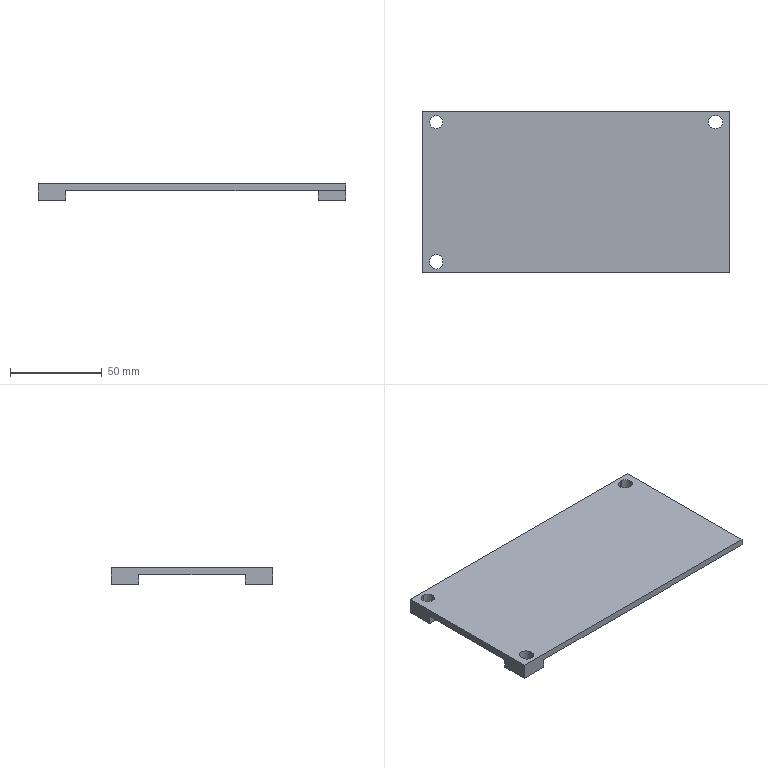Part | NX | 1 solid | 29 faces | box 168 x 88.2 x 8.8 mm | volume 57917 mm3 | plane 22 | cylinder 7 | commonest cylinder face diameters 7.17 x7
STEP:
#1=CARTESIAN_POINT('',(76.615,34.515,-8.8));
#2=VERTEX_POINT('',#1);
#3=CARTESIAN_POINT('',(76.615,34.515,0.));
#4=VERTEX_POINT('',#3);
#5=CARTESIAN_POINT('',(76.615,34.515,-8.8));
#6=DIRECTION('',(0.,0.,1.));
#7=VECTOR('',#6,1000.);
#8=LINE('',#5,#7);
#9=EDGE_CURVE('',#2,#4,#8,.T.);
#10=ORIENTED_EDGE('',*,*,#9,.T.);
#11=CARTESIAN_POINT('',(76.615,41.685,0.));
#12=VERTEX_POINT('',#11);
#13=CARTESIAN_POINT('',(76.615,38.1,0.));
#14=DIRECTION('',(0.,0.,-1.));
#15=DIRECTION('',(0.,1.,0.));
#16=AXIS2_PLACEMENT_3D('',#13,#14,#15);
#17=CIRCLE('',#16,3.585);
#18=EDGE_CURVE('',#12,#4,#17,.T.);
#19=ORIENTED_EDGE('',*,*,#18,.F.);
#20=CARTESIAN_POINT('',(76.615,41.685,-8.8));
#21=VERTEX_POINT('',#20);
#22=CARTESIAN_POINT('',(76.615,41.685,0.));
#23=DIRECTION('',(0.,0.,-1.));
#24=VECTOR('',#23,1000.);
#25=LINE('',#22,#24);
#26=EDGE_CURVE('',#12,#21,#25,.T.);
#27=ORIENTED_EDGE('',*,*,#26,.T.);
#28=CARTESIAN_POINT('',(76.615,38.1,-8.8));
#29=DIRECTION('',(0.,0.,1.));
#30=DIRECTION('',(0.,-1.,0.));
#31=AXIS2_PLACEMENT_3D('',#28,#29,#30);
#32=CIRCLE('',#31,3.585);
#33=EDGE_CURVE('',#2,#21,#32,.T.);
#34=ORIENTED_EDGE('',*,*,#33,.F.);
#35=EDGE_LOOP('',(#10,#19,#27,#34));
#36=FACE_BOUND('',#35,.T.);
#37=CARTESIAN_POINT('',(76.615,38.1,0.));
#38=DIRECTION('',(0.,0.,-1.));
#39=DIRECTION('',(0.,1.,0.));
#40=AXIS2_PLACEMENT_3D('',#37,#38,#39);
#41=CYLINDRICAL_SURFACE('',#40,3.585);
#42=ADVANCED_FACE('',(#36),#41,.F.);
#43=CARTESIAN_POINT('',(69.,29.1,-8.8));
#44=VERTEX_POINT('',#43);
#45=CARTESIAN_POINT('',(69.,44.1,-8.8));
#46=VERTEX_POINT('',#45);
#47=CARTESIAN_POINT('',(69.,29.1,-8.8));
#48=DIRECTION('',(0.,1.,0.));
#49=VECTOR('',#48,1000.);
#50=LINE('',#47,#49);
#51=EDGE_CURVE('',#44,#46,#50,.T.);
#52=ORIENTED_EDGE('',*,*,#51,.T.);
#53=CARTESIAN_POINT('',(84.,44.1,-8.8));
#54=VERTEX_POINT('',#53);
#55=CARTESIAN_POINT('',(84.,44.1,-8.8));
#56=DIRECTION('',(-1.,0.,0.));
#57=VECTOR('',#56,1000.);
#58=LINE('',#55,#57);
#59=EDGE_CURVE('',#54,#46,#58,.T.);
#60=ORIENTED_EDGE('',*,*,#59,.F.);
#61=CARTESIAN_POINT('',(84.,29.1,-8.8));
#62=VERTEX_POINT('',#61);
#63=CARTESIAN_POINT('',(84.,29.1,-8.8));
#64=DIRECTION('',(0.,1.,0.));
#65=VECTOR('',#64,1000.);
#66=LINE('',#63,#65);
#67=EDGE_CURVE('',#62,#54,#66,.T.);
#68=ORIENTED_EDGE('',*,*,#67,.F.);
#69=CARTESIAN_POINT('',(84.,29.1,-8.8));
#70=DIRECTION('',(-1.,0.,0.));
#71=VECTOR('',#70,1000.);
#72=LINE('',#69,#71);
#73=EDGE_CURVE('',#62,#44,#72,.T.);
#74=ORIENTED_EDGE('',*,*,#73,.T.);
#75=EDGE_LOOP('',(#52,#60,#68,#74));
#76=FACE_BOUND('',#75,.T.);
#77=CARTESIAN_POINT('',(75.785,41.685,-8.8));
#78=VERTEX_POINT('',#77);
#79=CARTESIAN_POINT('',(76.615,41.685,-8.8));
#80=DIRECTION('',(-1.,0.,0.));
#81=VECTOR('',#80,1000.);
#82=LINE('',#79,#81);
#83=EDGE_CURVE('',#21,#78,#82,.T.);
#84=ORIENTED_EDGE('',*,*,#83,.T.);
#85=CARTESIAN_POINT('',(75.785,34.515,-8.8));
#86=VERTEX_POINT('',#85);
#87=CARTESIAN_POINT('',(75.785,38.1,-8.8));
#88=DIRECTION('',(0.,0.,1.));
#89=DIRECTION('',(0.,1.,0.));
#90=AXIS2_PLACEMENT_3D('',#87,#88,#89);
#91=CIRCLE('',#90,3.585);
#92=EDGE_CURVE('',#78,#86,#91,.T.);
#93=ORIENTED_EDGE('',*,*,#92,.T.);
#94=CARTESIAN_POINT('',(75.785,34.515,-8.8));
#95=DIRECTION('',(1.,0.,0.));
#96=VECTOR('',#95,1000.);
#97=LINE('',#94,#96);
#98=EDGE_CURVE('',#86,#2,#97,.T.);
#99=ORIENTED_EDGE('',*,*,#98,.T.);
#100=ORIENTED_EDGE('',*,*,#33,.T.);
#101=EDGE_LOOP('',(#84,#93,#99,#100));
#102=FACE_BOUND('',#101,.T.);
#103=CARTESIAN_POINT('',(0.,0.,-8.8));
#104=DIRECTION('',(0.,0.,-1.));
#105=DIRECTION('',(0.,1.,0.));
#106=AXIS2_PLACEMENT_3D('',#103,#104,#105);
#107=PLANE('',#106);
#108=ADVANCED_FACE('',(#76,#102),#107,.T.);
#109=CARTESIAN_POINT('',(84.,29.1,-3.8));
#110=VERTEX_POINT('',#109);
#111=CARTESIAN_POINT('',(84.,29.1,-8.8));
#112=DIRECTION('',(0.,0.,1.));
#113=VECTOR('',#112,1000.);
#114=LINE('',#111,#113);
#115=EDGE_CURVE('',#62,#110,#114,.T.);
#116=ORIENTED_EDGE('',*,*,#115,.T.);
#117=CARTESIAN_POINT('',(69.,29.1,-3.8));
#118=VERTEX_POINT('',#117);
#119=CARTESIAN_POINT('',(84.,29.1,-3.8));
#120=DIRECTION('',(-1.,0.,0.));
#121=VECTOR('',#120,1000.);
#122=LINE('',#119,#121);
#123=EDGE_CURVE('',#110,#118,#122,.T.);
#124=ORIENTED_EDGE('',*,*,#123,.T.);
#125=CARTESIAN_POINT('',(69.,29.1,-8.8));
#126=DIRECTION('',(0.,0.,1.));
#127=VECTOR('',#126,1000.);
#128=LINE('',#125,#127);
#129=EDGE_CURVE('',#44,#118,#128,.T.);
#130=ORIENTED_EDGE('',*,*,#129,.F.);
#131=ORIENTED_EDGE('',*,*,#73,.F.);
#132=EDGE_LOOP('',(#116,#124,#130,#131));
#133=FACE_BOUND('',#132,.T.);
#134=CARTESIAN_POINT('',(84.,29.1,-3.8));
#135=DIRECTION('',(0.,1.,0.));
#136=DIRECTION('',(-1.,0.,0.));
#137=AXIS2_PLACEMENT_3D('',#134,#135,#136);
#138=PLANE('',#137);
#139=ADVANCED_FACE('',(#133),#138,.F.);
#140=ORIENTED_EDGE('',*,*,#129,.T.);
#141=CARTESIAN_POINT('',(69.,44.1,-3.8));
#142=VERTEX_POINT('',#141);
#143=CARTESIAN_POINT('',(69.,29.1,-3.8));
#144=DIRECTION('',(0.,1.,0.));
#145=VECTOR('',#144,1000.);
#146=LINE('',#143,#145);
#147=EDGE_CURVE('',#118,#142,#146,.T.);
#148=ORIENTED_EDGE('',*,*,#147,.T.);
#149=CARTESIAN_POINT('',(69.,44.1,-8.8));
#150=DIRECTION('',(0.,0.,1.));
#151=VECTOR('',#150,1000.);
#152=LINE('',#149,#151);
#153=EDGE_CURVE('',#46,#142,#152,.T.);
#154=ORIENTED_EDGE('',*,*,#153,.F.);
#155=ORIENTED_EDGE('',*,*,#51,.F.);
#156=EDGE_LOOP('',(#140,#148,#154,#155));
#157=FACE_BOUND('',#156,.T.);
#158=CARTESIAN_POINT('',(69.,44.1,-3.8));
#159=DIRECTION('',(1.,0.,0.));
#160=DIRECTION('',(0.,1.,0.));
#161=AXIS2_PLACEMENT_3D('',#158,#159,#160);
#162=PLANE('',#161);
#163=ADVANCED_FACE('',(#157),#162,.F.);
#164=ORIENTED_EDGE('',*,*,#153,.T.);
#165=CARTESIAN_POINT('',(-69.,44.1,-3.8));
#166=VERTEX_POINT('',#165);
#167=CARTESIAN_POINT('',(69.,44.1,-3.8));
#168=DIRECTION('',(-1.,0.,0.));
#169=VECTOR('',#168,1000.);
#170=LINE('',#167,#169);
#171=EDGE_CURVE('',#142,#166,#170,.T.);
#172=ORIENTED_EDGE('',*,*,#171,.T.);
#173=CARTESIAN_POINT('',(-69.,44.1,-8.8));
#174=VERTEX_POINT('',#173);
#175=CARTESIAN_POINT('',(-69.,44.1,-8.8));
#176=DIRECTION('',(0.,0.,1.));
#177=VECTOR('',#176,1000.);
#178=LINE('',#175,#177);
#179=EDGE_CURVE('',#174,#166,#178,.T.);
#180=ORIENTED_EDGE('',*,*,#179,.F.);
#181=CARTESIAN_POINT('',(-84.,44.1,-8.8));
#182=VERTEX_POINT('',#181);
#183=CARTESIAN_POINT('',(-69.,44.1,-8.8));
#184=DIRECTION('',(-1.,0.,0.));
#185=VECTOR('',#184,1000.);
#186=LINE('',#183,#185);
#187=EDGE_CURVE('',#174,#182,#186,.T.);
#188=ORIENTED_EDGE('',*,*,#187,.T.);
#189=CARTESIAN_POINT('',(-84.,44.1,0.));
#190=VERTEX_POINT('',#189);
#191=CARTESIAN_POINT('',(-84.,44.1,0.));
#192=DIRECTION('',(0.,0.,-1.));
#193=VECTOR('',#192,1000.);
#194=LINE('',#191,#193);
#195=EDGE_CURVE('',#190,#182,#194,.T.);
#196=ORIENTED_EDGE('',*,*,#195,.F.);
#197=CARTESIAN_POINT('',(84.,44.1,0.));
#198=VERTEX_POINT('',#197);
#199=CARTESIAN_POINT('',(84.,44.1,0.));
#200=DIRECTION('',(-1.,0.,0.));
#201=VECTOR('',#200,1000.);
#202=LINE('',#199,#201);
#203=EDGE_CURVE('',#198,#190,#202,.T.);
#204=ORIENTED_EDGE('',*,*,#203,.F.);
#205=CARTESIAN_POINT('',(84.,44.1,0.));
#206=DIRECTION('',(0.,0.,-1.));
#207=VECTOR('',#206,1000.);
#208=LINE('',#205,#207);
#209=EDGE_CURVE('',#198,#54,#208,.T.);
#210=ORIENTED_EDGE('',*,*,#209,.T.);
#211=ORIENTED_EDGE('',*,*,#59,.T.);
#212=EDGE_LOOP('',(#164,#172,#180,#188,#196,#204,#210,#211));
#213=FACE_BOUND('',#212,.T.);
#214=CARTESIAN_POINT('',(84.,44.1,-8.8));
#215=DIRECTION('',(0.,-1.,0.));
#216=DIRECTION('',(1.,0.,0.));
#217=AXIS2_PLACEMENT_3D('',#214,#215,#216);
#218=PLANE('',#217);
#219=ADVANCED_FACE('',(#213),#218,.F.);
#220=CARTESIAN_POINT('',(84.,9.867,-3.8));
#221=VERTEX_POINT('',#220);
#222=CARTESIAN_POINT('',(84.,9.867,-3.6));
#223=VERTEX_POINT('',#222);
#224=CARTESIAN_POINT('',(84.,9.867,-3.8));
#225=DIRECTION('',(0.,0.,1.));
#226=VECTOR('',#225,1000.);
#227=LINE('',#224,#226);
#228=EDGE_CURVE('',#221,#223,#227,.T.);
#229=ORIENTED_EDGE('',*,*,#228,.F.);
#230=CARTESIAN_POINT('',(84.,9.867,-3.8));
#231=DIRECTION('',(0.,1.,0.));
#232=VECTOR('',#231,1000.);
#233=LINE('',#230,#232);
#234=EDGE_CURVE('',#221,#110,#233,.T.);
#235=ORIENTED_EDGE('',*,*,#234,.T.);
#236=ORIENTED_EDGE('',*,*,#115,.F.);
#237=ORIENTED_EDGE('',*,*,#67,.T.);
#238=ORIENTED_EDGE('',*,*,#209,.F.);
#239=CARTESIAN_POINT('',(84.,-44.1,0.));
#240=VERTEX_POINT('',#239);
#241=CARTESIAN_POINT('',(84.,-44.1,0.));
#242=DIRECTION('',(0.,1.,0.));
#243=VECTOR('',#242,1000.);
#244=LINE('',#241,#243);
#245=EDGE_CURVE('',#240,#198,#244,.T.);
#246=ORIENTED_EDGE('',*,*,#245,.F.);
#247=CARTESIAN_POINT('',(84.,-44.1,-3.6));
#248=VERTEX_POINT('',#247);
#249=CARTESIAN_POINT('',(84.,-44.1,0.));
#250=DIRECTION('',(0.,0.,-1.));
#251=VECTOR('',#250,1000.);
#252=LINE('',#249,#251);
#253=EDGE_CURVE('',#240,#248,#252,.T.);
#254=ORIENTED_EDGE('',*,*,#253,.T.);
#255=CARTESIAN_POINT('',(84.,-44.1,-3.6));
#256=DIRECTION('',(0.,1.,0.));
#257=VECTOR('',#256,1000.);
#258=LINE('',#255,#257);
#259=EDGE_CURVE('',#248,#223,#258,.T.);
#260=ORIENTED_EDGE('',*,*,#259,.T.);
#261=EDGE_LOOP('',(#229,#235,#236,#237,#238,#246,#254,#260));
#262=FACE_BOUND('',#261,.T.);
#263=CARTESIAN_POINT('',(84.,44.1,-8.8));
#264=DIRECTION('',(-1.,0.,0.));
#265=DIRECTION('',(0.,-1.,0.));
#266=AXIS2_PLACEMENT_3D('',#263,#264,#265);
#267=PLANE('',#266);
#268=ADVANCED_FACE('',(#262),#267,.F.);
#269=ORIENTED_EDGE('',*,*,#259,.F.);
#270=CARTESIAN_POINT('',(28.934,-44.1,-3.6));
#271=VERTEX_POINT('',#270);
#272=CARTESIAN_POINT('',(28.934,-44.1,-3.6));
#273=DIRECTION('',(1.,0.,0.));
#274=VECTOR('',#273,1000.);
#275=LINE('',#272,#274);
#276=EDGE_CURVE('',#271,#248,#275,.T.);
#277=ORIENTED_EDGE('',*,*,#276,.F.);
#278=CARTESIAN_POINT('',(28.934,9.867,-3.6));
#279=VERTEX_POINT('',#278);
#280=CARTESIAN_POINT('',(28.934,9.867,-3.6));
#281=DIRECTION('',(0.,-1.,0.));
#282=VECTOR('',#281,1000.);
#283=LINE('',#280,#282);
#284=EDGE_CURVE('',#279,#271,#283,.T.);
#285=ORIENTED_EDGE('',*,*,#284,.F.);
#286=CARTESIAN_POINT('',(84.,9.867,-3.6));
#287=DIRECTION('',(-1.,0.,0.));
#288=VECTOR('',#287,1000.);
#289=LINE('',#286,#288);
#290=EDGE_CURVE('',#223,#279,#289,.T.);
#291=ORIENTED_EDGE('',*,*,#290,.F.);
#292=EDGE_LOOP('',(#269,#277,#285,#291));
#293=FACE_BOUND('',#292,.T.);
#294=CARTESIAN_POINT('',(0.,0.,-3.6));
#295=DIRECTION('',(0.,0.,-1.));
#296=DIRECTION('',(0.,1.,0.));
#297=AXIS2_PLACEMENT_3D('',#294,#295,#296);
#298=PLANE('',#297);
#299=ADVANCED_FACE('',(#293),#298,.T.);
#300=ORIENTED_EDGE('',*,*,#228,.T.);
#301=ORIENTED_EDGE('',*,*,#290,.T.);
#302=CARTESIAN_POINT('',(28.934,9.867,-3.8));
#303=VERTEX_POINT('',#302);
#304=CARTESIAN_POINT('',(28.934,9.867,-3.8));
#305=DIRECTION('',(0.,0.,1.));
#306=VECTOR('',#305,1000.);
#307=LINE('',#304,#306);
#308=EDGE_CURVE('',#303,#279,#307,.T.);
#309=ORIENTED_EDGE('',*,*,#308,.F.);
#310=CARTESIAN_POINT('',(84.,9.867,-3.8));
#311=DIRECTION('',(-1.,0.,0.));
#312=VECTOR('',#311,1000.);
#313=LINE('',#310,#312);
#314=EDGE_CURVE('',#221,#303,#313,.T.);
#315=ORIENTED_EDGE('',*,*,#314,.F.);
#316=EDGE_LOOP('',(#300,#301,#309,#315));
#317=FACE_BOUND('',#316,.T.);
#318=CARTESIAN_POINT('',(28.934,9.867,-3.6));
#319=DIRECTION('',(0.,1.,0.));
#320=DIRECTION('',(-1.,0.,0.));
#321=AXIS2_PLACEMENT_3D('',#318,#319,#320);
#322=PLANE('',#321);
#323=ADVANCED_FACE('',(#317),#322,.F.);
#324=CARTESIAN_POINT('',(28.934,-44.1,-3.8));
#325=VERTEX_POINT('',#324);
#326=CARTESIAN_POINT('',(28.934,9.867,-3.8));
#327=DIRECTION('',(0.,-1.,0.));
#328=VECTOR('',#327,1000.);
#329=LINE('',#326,#328);
#330=EDGE_CURVE('',#303,#325,#329,.T.);
#331=ORIENTED_EDGE('',*,*,#330,.T.);
#332=CARTESIAN_POINT('',(-69.,-44.1,-3.8));
#333=VERTEX_POINT('',#332);
#334=CARTESIAN_POINT('',(-69.,-44.1,-3.8));
#335=DIRECTION('',(1.,0.,0.));
#336=VECTOR('',#335,1000.);
#337=LINE('',#334,#336);
#338=EDGE_CURVE('',#333,#325,#337,.T.);
#339=ORIENTED_EDGE('',*,*,#338,.F.);
#340=CARTESIAN_POINT('',(-69.,-29.1,-3.8));
#341=VERTEX_POINT('',#340);
#342=CARTESIAN_POINT('',(-69.,-29.1,-3.8));
#343=DIRECTION('',(0.,-1.,0.));
#344=VECTOR('',#343,1000.);
#345=LINE('',#342,#344);
#346=EDGE_CURVE('',#341,#333,#345,.T.);
#347=ORIENTED_EDGE('',*,*,#346,.F.);
#348=CARTESIAN_POINT('',(-84.,-29.1,-3.8));
#349=VERTEX_POINT('',#348);
#350=CARTESIAN_POINT('',(-84.,-29.1,-3.8));
#351=DIRECTION('',(1.,0.,0.));
#352=VECTOR('',#351,1000.);
#353=LINE('',#350,#352);
#354=EDGE_CURVE('',#349,#341,#353,.T.);
#355=ORIENTED_EDGE('',*,*,#354,.F.);
#356=CARTESIAN_POINT('',(-84.,29.1,-3.8));
#357=VERTEX_POINT('',#356);
#358=CARTESIAN_POINT('',(-84.,29.1,-3.8));
#359=DIRECTION('',(0.,-1.,0.));
#360=VECTOR('',#359,1000.);
#361=LINE('',#358,#360);
#362=EDGE_CURVE('',#357,#349,#361,.T.);
#363=ORIENTED_EDGE('',*,*,#362,.F.);
#364=CARTESIAN_POINT('',(-69.,29.1,-3.8));
#365=VERTEX_POINT('',#364);
#366=CARTESIAN_POINT('',(-69.,29.1,-3.8));
#367=DIRECTION('',(-1.,0.,0.));
#368=VECTOR('',#367,1000.);
#369=LINE('',#366,#368);
#370=EDGE_CURVE('',#365,#357,#369,.T.);
#371=ORIENTED_EDGE('',*,*,#370,.F.);
#372=CARTESIAN_POINT('',(-69.,44.1,-3.8));
#373=DIRECTION('',(0.,-1.,0.));
#374=VECTOR('',#373,1000.);
#375=LINE('',#372,#374);
#376=EDGE_CURVE('',#166,#365,#375,.T.);
#377=ORIENTED_EDGE('',*,*,#376,.F.);
#378=ORIENTED_EDGE('',*,*,#171,.F.);
#379=ORIENTED_EDGE('',*,*,#147,.F.);
#380=ORIENTED_EDGE('',*,*,#123,.F.);
#381=ORIENTED_EDGE('',*,*,#234,.F.);
#382=ORIENTED_EDGE('',*,*,#314,.T.);
#383=EDGE_LOOP('',(#331,#339,#347,#355,#363,#371,#377,#378,#379,#380,#381,#382));
#384=FACE_BOUND('',#383,.T.);
#385=CARTESIAN_POINT('',(0.,0.,-3.8));
#386=DIRECTION('',(0.,0.,-1.));
#387=DIRECTION('',(0.,1.,0.));
#388=AXIS2_PLACEMENT_3D('',#385,#386,#387);
#389=PLANE('',#388);
#390=ADVANCED_FACE('',(#384),#389,.T.);
#391=ORIENTED_EDGE('',*,*,#179,.T.);
#392=ORIENTED_EDGE('',*,*,#376,.T.);
#393=CARTESIAN_POINT('',(-69.,29.1,-8.8));
#394=VERTEX_POINT('',#393);
#395=CARTESIAN_POINT('',(-69.,29.1,-8.8));
#396=DIRECTION('',(0.,0.,1.));
#397=VECTOR('',#396,1000.);
#398=LINE('',#395,#397);
#399=EDGE_CURVE('',#394,#365,#398,.T.);
#400=ORIENTED_EDGE('',*,*,#399,.F.);
#401=CARTESIAN_POINT('',(-69.,44.1,-8.8));
#402=DIRECTION('',(0.,-1.,0.));
#403=VECTOR('',#402,1000.);
#404=LINE('',#401,#403);
#405=EDGE_CURVE('',#174,#394,#404,.T.);
#406=ORIENTED_EDGE('',*,*,#405,.F.);
#407=EDGE_LOOP('',(#391,#392,#400,#406));
#408=FACE_BOUND('',#407,.T.);
#409=CARTESIAN_POINT('',(-69.,44.1,-3.8));
#410=DIRECTION('',(-1.,0.,0.));
#411=DIRECTION('',(0.,-1.,0.));
#412=AXIS2_PLACEMENT_3D('',#409,#410,#411);
#413=PLANE('',#412);
#414=ADVANCED_FACE('',(#408),#413,.F.);
#415=CARTESIAN_POINT('',(-84.,29.1,-8.8));
#416=VERTEX_POINT('',#415);
#417=CARTESIAN_POINT('',(-69.,29.1,-8.8));
#418=DIRECTION('',(-1.,0.,0.));
#419=VECTOR('',#418,1000.);
#420=LINE('',#417,#419);
#421=EDGE_CURVE('',#394,#416,#420,.T.);
#422=ORIENTED_EDGE('',*,*,#421,.T.);
#423=CARTESIAN_POINT('',(-84.,44.1,-8.8));
#424=DIRECTION('',(0.,-1.,0.));
#425=VECTOR('',#424,1000.);
#426=LINE('',#423,#425);
#427=EDGE_CURVE('',#182,#416,#426,.T.);
#428=ORIENTED_EDGE('',*,*,#427,.F.);
#429=ORIENTED_EDGE('',*,*,#187,.F.);
#430=ORIENTED_EDGE('',*,*,#405,.T.);
#431=EDGE_LOOP('',(#422,#428,#429,#430));
#432=FACE_BOUND('',#431,.T.);
#433=CARTESIAN_POINT('',(-76.2,34.515,-8.8));
#434=VERTEX_POINT('',#433);
#435=CARTESIAN_POINT('',(-76.2,41.685,-8.8));
#436=VERTEX_POINT('',#435);
#437=CARTESIAN_POINT('',(-76.2,38.1,-8.8));
#438=DIRECTION('',(0.,0.,1.));
#439=DIRECTION('',(0.,-1.,0.));
#440=AXIS2_PLACEMENT_3D('',#437,#438,#439);
#441=CIRCLE('',#440,3.585);
#442=EDGE_CURVE('',#434,#436,#441,.T.);
#443=ORIENTED_EDGE('',*,*,#442,.T.);
#444=CARTESIAN_POINT('',(-76.2,38.1,-8.8));
#445=DIRECTION('',(0.,0.,1.));
#446=DIRECTION('',(0.,1.,0.));
#447=AXIS2_PLACEMENT_3D('',#444,#445,#446);
#448=CIRCLE('',#447,3.585);
#449=EDGE_CURVE('',#436,#434,#448,.T.);
#450=ORIENTED_EDGE('',*,*,#449,.T.);
#451=EDGE_LOOP('',(#443,#450));
#452=FACE_BOUND('',#451,.T.);
#453=CARTESIAN_POINT('',(0.,0.,-8.8));
#454=DIRECTION('',(0.,0.,-1.));
#455=DIRECTION('',(0.,1.,0.));
#456=AXIS2_PLACEMENT_3D('',#453,#454,#455);
#457=PLANE('',#456);
#458=ADVANCED_FACE('',(#432,#452),#457,.T.);
#459=CARTESIAN_POINT('',(-84.,29.1,-8.8));
#460=DIRECTION('',(0.,0.,1.));
#461=VECTOR('',#460,1000.);
#462=LINE('',#459,#461);
#463=EDGE_CURVE('',#416,#357,#462,.T.);
#464=ORIENTED_EDGE('',*,*,#463,.T.);
#465=ORIENTED_EDGE('',*,*,#362,.T.);
#466=CARTESIAN_POINT('',(-84.,-29.1,-8.8));
#467=VERTEX_POINT('',#466);
#468=CARTESIAN_POINT('',(-84.,-29.1,-8.8));
#469=DIRECTION('',(0.,0.,1.));
#470=VECTOR('',#469,1000.);
#471=LINE('',#468,#470);
#472=EDGE_CURVE('',#467,#349,#471,.T.);
#473=ORIENTED_EDGE('',*,*,#472,.F.);
#474=CARTESIAN_POINT('',(-84.,-44.1,-8.8));
#475=VERTEX_POINT('',#474);
#476=CARTESIAN_POINT('',(-84.,-29.1,-8.8));
#477=DIRECTION('',(0.,-1.,0.));
#478=VECTOR('',#477,1000.);
#479=LINE('',#476,#478);
#480=EDGE_CURVE('',#467,#475,#479,.T.);
#481=ORIENTED_EDGE('',*,*,#480,.T.);
#482=CARTESIAN_POINT('',(-84.,-44.1,0.));
#483=VERTEX_POINT('',#482);
#484=CARTESIAN_POINT('',(-84.,-44.1,0.));
#485=DIRECTION('',(0.,0.,-1.));
#486=VECTOR('',#485,1000.);
#487=LINE('',#484,#486);
#488=EDGE_CURVE('',#483,#475,#487,.T.);
#489=ORIENTED_EDGE('',*,*,#488,.F.);
#490=CARTESIAN_POINT('',(-84.,44.1,0.));
#491=DIRECTION('',(0.,-1.,0.));
#492=VECTOR('',#491,1000.);
#493=LINE('',#490,#492);
#494=EDGE_CURVE('',#190,#483,#493,.T.);
#495=ORIENTED_EDGE('',*,*,#494,.F.);
#496=ORIENTED_EDGE('',*,*,#195,.T.);
#497=ORIENTED_EDGE('',*,*,#427,.T.);
#498=EDGE_LOOP('',(#464,#465,#473,#481,#489,#495,#496,#497));
#499=FACE_BOUND('',#498,.T.);
#500=CARTESIAN_POINT('',(-84.,44.1,-8.8));
#501=DIRECTION('',(1.,0.,0.));
#502=DIRECTION('',(0.,1.,0.));
#503=AXIS2_PLACEMENT_3D('',#500,#501,#502);
#504=PLANE('',#503);
#505=ADVANCED_FACE('',(#499),#504,.F.);
#506=CARTESIAN_POINT('',(-84.,-44.1,0.));
#507=DIRECTION('',(1.,0.,0.));
#508=VECTOR('',#507,1000.);
#509=LINE('',#506,#508);
#510=EDGE_CURVE('',#483,#240,#509,.T.);
#511=ORIENTED_EDGE('',*,*,#510,.T.);
#512=ORIENTED_EDGE('',*,*,#245,.T.);
#513=ORIENTED_EDGE('',*,*,#203,.T.);
#514=ORIENTED_EDGE('',*,*,#494,.T.);
#515=EDGE_LOOP('',(#511,#512,#513,#514));
#516=FACE_BOUND('',#515,.T.);
#517=ORIENTED_EDGE('',*,*,#18,.T.);
#518=CARTESIAN_POINT('',(75.785,34.515,0.));
#519=VERTEX_POINT('',#518);
#520=CARTESIAN_POINT('',(75.785,34.515,0.));
#521=DIRECTION('',(1.,0.,0.));
#522=VECTOR('',#521,1000.);
#523=LINE('',#520,#522);
#524=EDGE_CURVE('',#519,#4,#523,.T.);
#525=ORIENTED_EDGE('',*,*,#524,.F.);
#526=CARTESIAN_POINT('',(75.785,41.685,0.));
#527=VERTEX_POINT('',#526);
#528=CARTESIAN_POINT('',(75.785,38.1,0.));
#529=DIRECTION('',(0.,0.,-1.));
#530=DIRECTION('',(0.,-1.,0.));
#531=AXIS2_PLACEMENT_3D('',#528,#529,#530);
#532=CIRCLE('',#531,3.585);
#533=EDGE_CURVE('',#519,#527,#532,.T.);
#534=ORIENTED_EDGE('',*,*,#533,.T.);
#535=CARTESIAN_POINT('',(76.615,41.685,0.));
#536=DIRECTION('',(-1.,0.,0.));
#537=VECTOR('',#536,1000.);
#538=LINE('',#535,#537);
#539=EDGE_CURVE('',#12,#527,#538,.T.);
#540=ORIENTED_EDGE('',*,*,#539,.F.);
#541=EDGE_LOOP('',(#517,#525,#534,#540));
#542=FACE_BOUND('',#541,.T.);
#543=CARTESIAN_POINT('',(-79.785,-37.685,0.));
#544=VERTEX_POINT('',#543);
#545=CARTESIAN_POINT('',(-76.2,-34.1,0.));
#546=VERTEX_POINT('',#545);
#547=CARTESIAN_POINT('',(-76.2,-37.685,0.));
#548=DIRECTION('',(0.,0.,-1.));
#549=DIRECTION('',(-1.,0.,0.));
#550=AXIS2_PLACEMENT_3D('',#547,#548,#549);
#551=CIRCLE('',#550,3.585);
#552=EDGE_CURVE('',#544,#546,#551,.T.);
#553=ORIENTED_EDGE('',*,*,#552,.T.);
#554=CARTESIAN_POINT('',(-72.615,-37.685,0.));
#555=VERTEX_POINT('',#554);
#556=CARTESIAN_POINT('',(-76.2,-37.685,0.));
#557=DIRECTION('',(0.,0.,-1.));
#558=DIRECTION('',(0.,1.,0.));
#559=AXIS2_PLACEMENT_3D('',#556,#557,#558);
#560=CIRCLE('',#559,3.585);
#561=EDGE_CURVE('',#546,#555,#560,.T.);
#562=ORIENTED_EDGE('',*,*,#561,.T.);
#563=CARTESIAN_POINT('',(-72.615,-38.515,0.));
#564=VERTEX_POINT('',#563);
#565=CARTESIAN_POINT('',(-72.615,-38.515,0.));
#566=DIRECTION('',(0.,1.,0.));
#567=VECTOR('',#566,1000.);
#568=LINE('',#565,#567);
#569=EDGE_CURVE('',#564,#555,#568,.T.);
#570=ORIENTED_EDGE('',*,*,#569,.F.);
#571=CARTESIAN_POINT('',(-76.2,-42.1,0.));
#572=VERTEX_POINT('',#571);
#573=CARTESIAN_POINT('',(-76.2,-38.515,0.));
#574=DIRECTION('',(0.,0.,-1.));
#575=DIRECTION('',(1.,0.,0.));
#576=AXIS2_PLACEMENT_3D('',#573,#574,#575);
#577=CIRCLE('',#576,3.585);
#578=EDGE_CURVE('',#564,#572,#577,.T.);
#579=ORIENTED_EDGE('',*,*,#578,.T.);
#580=CARTESIAN_POINT('',(-79.785,-38.515,0.));
#581=VERTEX_POINT('',#580);
#582=CARTESIAN_POINT('',(-76.2,-38.515,0.));
#583=DIRECTION('',(0.,0.,-1.));
#584=DIRECTION('',(0.,-1.,0.));
#585=AXIS2_PLACEMENT_3D('',#582,#583,#584);
#586=CIRCLE('',#585,3.585);
#587=EDGE_CURVE('',#572,#581,#586,.T.);
#588=ORIENTED_EDGE('',*,*,#587,.T.);
#589=CARTESIAN_POINT('',(-79.785,-37.685,0.));
#590=DIRECTION('',(0.,-1.,0.));
#591=VECTOR('',#590,1000.);
#592=LINE('',#589,#591);
#593=EDGE_CURVE('',#544,#581,#592,.T.);
#594=ORIENTED_EDGE('',*,*,#593,.F.);
#595=EDGE_LOOP('',(#553,#562,#570,#579,#588,#594));
#596=FACE_BOUND('',#595,.T.);
#597=CARTESIAN_POINT('',(-76.2,41.685,0.));
#598=VERTEX_POINT('',#597);
#599=CARTESIAN_POINT('',(-76.2,34.515,0.));
#600=VERTEX_POINT('',#599);
#601=CARTESIAN_POINT('',(-76.2,38.1,0.));
#602=DIRECTION('',(0.,0.,-1.));
#603=DIRECTION('',(0.,1.,0.));
#604=AXIS2_PLACEMENT_3D('',#601,#602,#603);
#605=CIRCLE('',#604,3.585);
#606=EDGE_CURVE('',#598,#600,#605,.T.);
#607=ORIENTED_EDGE('',*,*,#606,.T.);
#608=CARTESIAN_POINT('',(-76.2,38.1,0.));
#609=DIRECTION('',(0.,0.,-1.));
#610=DIRECTION('',(0.,-1.,0.));
#611=AXIS2_PLACEMENT_3D('',#608,#609,#610);
#612=CIRCLE('',#611,3.585);
#613=EDGE_CURVE('',#600,#598,#612,.T.);
#614=ORIENTED_EDGE('',*,*,#613,.T.);
#615=EDGE_LOOP('',(#607,#614));
#616=FACE_BOUND('',#615,.T.);
#617=CARTESIAN_POINT('',(0.,0.,0.));
#618=DIRECTION('',(0.,0.,-1.));
#619=DIRECTION('',(0.,1.,0.));
#620=AXIS2_PLACEMENT_3D('',#617,#618,#619);
#621=PLANE('',#620);
#622=ADVANCED_FACE('',(#516,#542,#596,#616),#621,.F.);
#623=CARTESIAN_POINT('',(28.934,-44.1,-3.8));
#624=DIRECTION('',(0.,0.,1.));
#625=VECTOR('',#624,1000.);
#626=LINE('',#623,#625);
#627=EDGE_CURVE('',#325,#271,#626,.T.);
#628=ORIENTED_EDGE('',*,*,#627,.T.);
#629=ORIENTED_EDGE('',*,*,#276,.T.);
#630=ORIENTED_EDGE('',*,*,#253,.F.);
#631=ORIENTED_EDGE('',*,*,#510,.F.);
#632=ORIENTED_EDGE('',*,*,#488,.T.);
#633=CARTESIAN_POINT('',(-69.,-44.1,-8.8));
#634=VERTEX_POINT('',#633);
#635=CARTESIAN_POINT('',(-84.,-44.1,-8.8));
#636=DIRECTION('',(1.,0.,0.));
#637=VECTOR('',#636,1000.);
#638=LINE('',#635,#637);
#639=EDGE_CURVE('',#475,#634,#638,.T.);
#640=ORIENTED_EDGE('',*,*,#639,.T.);
#641=CARTESIAN_POINT('',(-69.,-44.1,-8.8));
#642=DIRECTION('',(0.,0.,1.));
#643=VECTOR('',#642,1000.);
#644=LINE('',#641,#643);
#645=EDGE_CURVE('',#634,#333,#644,.T.);
#646=ORIENTED_EDGE('',*,*,#645,.T.);
#647=ORIENTED_EDGE('',*,*,#338,.T.);
#648=EDGE_LOOP('',(#628,#629,#630,#631,#632,#640,#646,#647));
#649=FACE_BOUND('',#648,.T.);
#650=CARTESIAN_POINT('',(84.,-44.1,-8.8));
#651=DIRECTION('',(0.,1.,0.));
#652=DIRECTION('',(-1.,0.,0.));
#653=AXIS2_PLACEMENT_3D('',#650,#651,#652);
#654=PLANE('',#653);
#655=ADVANCED_FACE('',(#649),#654,.F.);
#656=CARTESIAN_POINT('',(-69.,-29.1,-8.8));
#657=VERTEX_POINT('',#656);
#658=CARTESIAN_POINT('',(-69.,-29.1,-8.8));
#659=DIRECTION('',(0.,0.,1.));
#660=VECTOR('',#659,1000.);
#661=LINE('',#658,#660);
#662=EDGE_CURVE('',#657,#341,#661,.T.);
#663=ORIENTED_EDGE('',*,*,#662,.T.);
#664=ORIENTED_EDGE('',*,*,#346,.T.);
#665=ORIENTED_EDGE('',*,*,#645,.F.);
#666=CARTESIAN_POINT('',(-69.,-29.1,-8.8));
#667=DIRECTION('',(0.,-1.,0.));
#668=VECTOR('',#667,1000.);
#669=LINE('',#666,#668);
#670=EDGE_CURVE('',#657,#634,#669,.T.);
#671=ORIENTED_EDGE('',*,*,#670,.F.);
#672=EDGE_LOOP('',(#663,#664,#665,#671));
#673=FACE_BOUND('',#672,.T.);
#674=CARTESIAN_POINT('',(-69.,-44.1,-3.8));
#675=DIRECTION('',(-1.,0.,0.));
#676=DIRECTION('',(0.,-1.,0.));
#677=AXIS2_PLACEMENT_3D('',#674,#675,#676);
#678=PLANE('',#677);
#679=ADVANCED_FACE('',(#673),#678,.F.);
#680=ORIENTED_EDGE('',*,*,#670,.T.);
#681=ORIENTED_EDGE('',*,*,#639,.F.);
#682=ORIENTED_EDGE('',*,*,#480,.F.);
#683=CARTESIAN_POINT('',(-84.,-29.1,-8.8));
#684=DIRECTION('',(1.,0.,0.));
#685=VECTOR('',#684,1000.);
#686=LINE('',#683,#685);
#687=EDGE_CURVE('',#467,#657,#686,.T.);
#688=ORIENTED_EDGE('',*,*,#687,.T.);
#689=EDGE_LOOP('',(#680,#681,#682,#688));
#690=FACE_BOUND('',#689,.T.);
#691=CARTESIAN_POINT('',(-76.2,-34.1,-8.8));
#692=VERTEX_POINT('',#691);
#693=CARTESIAN_POINT('',(-79.785,-37.685,-8.8));
#694=VERTEX_POINT('',#693);
#695=CARTESIAN_POINT('',(-76.2,-37.685,-8.8));
#696=DIRECTION('',(0.,0.,1.));
#697=DIRECTION('',(0.,1.,0.));
#698=AXIS2_PLACEMENT_3D('',#695,#696,#697);
#699=CIRCLE('',#698,3.585);
#700=EDGE_CURVE('',#692,#694,#699,.T.);
#701=ORIENTED_EDGE('',*,*,#700,.T.);
#702=CARTESIAN_POINT('',(-79.785,-38.515,-8.8));
#703=VERTEX_POINT('',#702);
#704=CARTESIAN_POINT('',(-79.785,-37.685,-8.8));
#705=DIRECTION('',(0.,-1.,0.));
#706=VECTOR('',#705,1000.);
#707=LINE('',#704,#706);
#708=EDGE_CURVE('',#694,#703,#707,.T.);
#709=ORIENTED_EDGE('',*,*,#708,.T.);
#710=CARTESIAN_POINT('',(-76.2,-42.1,-8.8));
#711=VERTEX_POINT('',#710);
#712=CARTESIAN_POINT('',(-76.2,-38.515,-8.8));
#713=DIRECTION('',(0.,0.,1.));
#714=DIRECTION('',(-1.,0.,0.));
#715=AXIS2_PLACEMENT_3D('',#712,#713,#714);
#716=CIRCLE('',#715,3.585);
#717=EDGE_CURVE('',#703,#711,#716,.T.);
#718=ORIENTED_EDGE('',*,*,#717,.T.);
#719=CARTESIAN_POINT('',(-72.615,-38.515,-8.8));
#720=VERTEX_POINT('',#719);
#721=CARTESIAN_POINT('',(-76.2,-38.515,-8.8));
#722=DIRECTION('',(0.,0.,1.));
#723=DIRECTION('',(0.,-1.,0.));
#724=AXIS2_PLACEMENT_3D('',#721,#722,#723);
#725=CIRCLE('',#724,3.585);
#726=EDGE_CURVE('',#711,#720,#725,.T.);
#727=ORIENTED_EDGE('',*,*,#726,.T.);
#728=CARTESIAN_POINT('',(-72.615,-37.685,-8.8));
#729=VERTEX_POINT('',#728);
#730=CARTESIAN_POINT('',(-72.615,-38.515,-8.8));
#731=DIRECTION('',(0.,1.,0.));
#732=VECTOR('',#731,1000.);
#733=LINE('',#730,#732);
#734=EDGE_CURVE('',#720,#729,#733,.T.);
#735=ORIENTED_EDGE('',*,*,#734,.T.);
#736=CARTESIAN_POINT('',(-76.2,-37.685,-8.8));
#737=DIRECTION('',(0.,0.,1.));
#738=DIRECTION('',(1.,0.,0.));
#739=AXIS2_PLACEMENT_3D('',#736,#737,#738);
#740=CIRCLE('',#739,3.585);
#741=EDGE_CURVE('',#729,#692,#740,.T.);
#742=ORIENTED_EDGE('',*,*,#741,.T.);
#743=EDGE_LOOP('',(#701,#709,#718,#727,#735,#742));
#744=FACE_BOUND('',#743,.T.);
#745=CARTESIAN_POINT('',(0.,0.,-8.8));
#746=DIRECTION('',(0.,0.,-1.));
#747=DIRECTION('',(0.,1.,0.));
#748=AXIS2_PLACEMENT_3D('',#745,#746,#747);
#749=PLANE('',#748);
#750=ADVANCED_FACE('',(#690,#744),#749,.T.);
#751=ORIENTED_EDGE('',*,*,#472,.T.);
#752=ORIENTED_EDGE('',*,*,#354,.T.);
#753=ORIENTED_EDGE('',*,*,#662,.F.);
#754=ORIENTED_EDGE('',*,*,#687,.F.);
#755=EDGE_LOOP('',(#751,#752,#753,#754));
#756=FACE_BOUND('',#755,.T.);
#757=CARTESIAN_POINT('',(-84.,-29.1,-3.8));
#758=DIRECTION('',(0.,-1.,0.));
#759=DIRECTION('',(1.,0.,0.));
#760=AXIS2_PLACEMENT_3D('',#757,#758,#759);
#761=PLANE('',#760);
#762=ADVANCED_FACE('',(#756),#761,.F.);
#763=ORIENTED_EDGE('',*,*,#741,.F.);
#764=CARTESIAN_POINT('',(-72.615,-37.685,-8.8));
#765=DIRECTION('',(0.,0.,1.));
#766=VECTOR('',#765,1000.);
#767=LINE('',#764,#766);
#768=EDGE_CURVE('',#729,#555,#767,.T.);
#769=ORIENTED_EDGE('',*,*,#768,.T.);
#770=ORIENTED_EDGE('',*,*,#561,.F.);
#771=ORIENTED_EDGE('',*,*,#552,.F.);
#772=CARTESIAN_POINT('',(-79.785,-37.685,0.));
#773=DIRECTION('',(0.,0.,-1.));
#774=VECTOR('',#773,1000.);
#775=LINE('',#772,#774);
#776=EDGE_CURVE('',#544,#694,#775,.T.);
#777=ORIENTED_EDGE('',*,*,#776,.T.);
#778=ORIENTED_EDGE('',*,*,#700,.F.);
#779=EDGE_LOOP('',(#763,#769,#770,#771,#777,#778));
#780=FACE_BOUND('',#779,.T.);
#781=CARTESIAN_POINT('',(-76.2,-37.685,0.));
#782=DIRECTION('',(0.,0.,-1.));
#783=DIRECTION('',(0.,1.,0.));
#784=AXIS2_PLACEMENT_3D('',#781,#782,#783);
#785=CYLINDRICAL_SURFACE('',#784,3.585);
#786=ADVANCED_FACE('',(#780),#785,.F.);
#787=ORIENTED_EDGE('',*,*,#776,.F.);
#788=ORIENTED_EDGE('',*,*,#593,.T.);
#789=CARTESIAN_POINT('',(-79.785,-38.515,-8.8));
#790=DIRECTION('',(0.,0.,1.));
#791=VECTOR('',#790,1000.);
#792=LINE('',#789,#791);
#793=EDGE_CURVE('',#703,#581,#792,.T.);
#794=ORIENTED_EDGE('',*,*,#793,.F.);
#795=ORIENTED_EDGE('',*,*,#708,.F.);
#796=EDGE_LOOP('',(#787,#788,#794,#795));
#797=FACE_BOUND('',#796,.T.);
#798=CARTESIAN_POINT('',(-79.785,-37.685,0.));
#799=DIRECTION('',(-1.,0.,0.));
#800=DIRECTION('',(0.,-1.,0.));
#801=AXIS2_PLACEMENT_3D('',#798,#799,#800);
#802=PLANE('',#801);
#803=ADVANCED_FACE('',(#797),#802,.F.);
#804=CARTESIAN_POINT('',(-76.2,-42.1,-8.8));
#805=DIRECTION('',(0.,0.,1.));
#806=VECTOR('',#805,1000.);
#807=LINE('',#804,#806);
#808=EDGE_CURVE('',#711,#572,#807,.T.);
#809=ORIENTED_EDGE('',*,*,#808,.F.);
#810=ORIENTED_EDGE('',*,*,#717,.F.);
#811=ORIENTED_EDGE('',*,*,#793,.T.);
#812=ORIENTED_EDGE('',*,*,#587,.F.);
#813=EDGE_LOOP('',(#809,#810,#811,#812));
#814=FACE_BOUND('',#813,.T.);
#815=CARTESIAN_POINT('',(-76.2,-38.515,0.));
#816=DIRECTION('',(0.,0.,-1.));
#817=DIRECTION('',(0.,1.,0.));
#818=AXIS2_PLACEMENT_3D('',#815,#816,#817);
#819=CYLINDRICAL_SURFACE('',#818,3.585);
#820=ADVANCED_FACE('',(#814),#819,.F.);
#821=ORIENTED_EDGE('',*,*,#578,.F.);
#822=CARTESIAN_POINT('',(-72.615,-38.515,0.));
#823=DIRECTION('',(0.,0.,-1.));
#824=VECTOR('',#823,1000.);
#825=LINE('',#822,#824);
#826=EDGE_CURVE('',#564,#720,#825,.T.);
#827=ORIENTED_EDGE('',*,*,#826,.T.);
#828=ORIENTED_EDGE('',*,*,#726,.F.);
#829=ORIENTED_EDGE('',*,*,#808,.T.);
#830=EDGE_LOOP('',(#821,#827,#828,#829));
#831=FACE_BOUND('',#830,.T.);
#832=CARTESIAN_POINT('',(-76.2,-38.515,0.));
#833=DIRECTION('',(0.,0.,-1.));
#834=DIRECTION('',(0.,1.,0.));
#835=AXIS2_PLACEMENT_3D('',#832,#833,#834);
#836=CYLINDRICAL_SURFACE('',#835,3.585);
#837=ADVANCED_FACE('',(#831),#836,.F.);
#838=ORIENTED_EDGE('',*,*,#826,.F.);
#839=ORIENTED_EDGE('',*,*,#569,.T.);
#840=ORIENTED_EDGE('',*,*,#768,.F.);
#841=ORIENTED_EDGE('',*,*,#734,.F.);
#842=EDGE_LOOP('',(#838,#839,#840,#841));
#843=FACE_BOUND('',#842,.T.);
#844=CARTESIAN_POINT('',(-72.615,-37.685,0.));
#845=DIRECTION('',(1.,0.,0.));
#846=DIRECTION('',(0.,1.,0.));
#847=AXIS2_PLACEMENT_3D('',#844,#845,#846);
#848=PLANE('',#847);
#849=ADVANCED_FACE('',(#843),#848,.F.);
#850=ORIENTED_EDGE('',*,*,#308,.T.);
#851=ORIENTED_EDGE('',*,*,#284,.T.);
#852=ORIENTED_EDGE('',*,*,#627,.F.);
#853=ORIENTED_EDGE('',*,*,#330,.F.);
#854=EDGE_LOOP('',(#850,#851,#852,#853));
#855=FACE_BOUND('',#854,.T.);
#856=CARTESIAN_POINT('',(28.934,-44.1,-3.6));
#857=DIRECTION('',(-1.,0.,0.));
#858=DIRECTION('',(0.,-1.,0.));
#859=AXIS2_PLACEMENT_3D('',#856,#857,#858);
#860=PLANE('',#859);
#861=ADVANCED_FACE('',(#855),#860,.F.);
#862=ORIENTED_EDGE('',*,*,#26,.F.);
#863=ORIENTED_EDGE('',*,*,#539,.T.);
#864=CARTESIAN_POINT('',(75.785,41.685,-8.8));
#865=DIRECTION('',(0.,0.,1.));
#866=VECTOR('',#865,1000.);
#867=LINE('',#864,#866);
#868=EDGE_CURVE('',#78,#527,#867,.T.);
#869=ORIENTED_EDGE('',*,*,#868,.F.);
#870=ORIENTED_EDGE('',*,*,#83,.F.);
#871=EDGE_LOOP('',(#862,#863,#869,#870));
#872=FACE_BOUND('',#871,.T.);
#873=CARTESIAN_POINT('',(76.615,41.685,0.));
#874=DIRECTION('',(0.,1.,0.));
#875=DIRECTION('',(-1.,0.,0.));
#876=AXIS2_PLACEMENT_3D('',#873,#874,#875);
#877=PLANE('',#876);
#878=ADVANCED_FACE('',(#872),#877,.F.);
#879=ORIENTED_EDGE('',*,*,#868,.T.);
#880=ORIENTED_EDGE('',*,*,#533,.F.);
#881=CARTESIAN_POINT('',(75.785,34.515,0.));
#882=DIRECTION('',(0.,0.,-1.));
#883=VECTOR('',#882,1000.);
#884=LINE('',#881,#883);
#885=EDGE_CURVE('',#519,#86,#884,.T.);
#886=ORIENTED_EDGE('',*,*,#885,.T.);
#887=ORIENTED_EDGE('',*,*,#92,.F.);
#888=EDGE_LOOP('',(#879,#880,#886,#887));
#889=FACE_BOUND('',#888,.T.);
#890=CARTESIAN_POINT('',(75.785,38.1,0.));
#891=DIRECTION('',(0.,0.,-1.));
#892=DIRECTION('',(0.,1.,0.));
#893=AXIS2_PLACEMENT_3D('',#890,#891,#892);
#894=CYLINDRICAL_SURFACE('',#893,3.585);
#895=ADVANCED_FACE('',(#889),#894,.F.);
#896=ORIENTED_EDGE('',*,*,#885,.F.);
#897=ORIENTED_EDGE('',*,*,#524,.T.);
#898=ORIENTED_EDGE('',*,*,#9,.F.);
#899=ORIENTED_EDGE('',*,*,#98,.F.);
#900=EDGE_LOOP('',(#896,#897,#898,#899));
#901=FACE_BOUND('',#900,.T.);
#902=CARTESIAN_POINT('',(76.615,34.515,0.));
#903=DIRECTION('',(0.,-1.,0.));
#904=DIRECTION('',(1.,0.,0.));
#905=AXIS2_PLACEMENT_3D('',#902,#903,#904);
#906=PLANE('',#905);
#907=ADVANCED_FACE('',(#901),#906,.F.);
#908=ORIENTED_EDGE('',*,*,#613,.F.);
#909=CARTESIAN_POINT('',(-76.2,34.515,-8.8));
#910=DIRECTION('',(0.,0.,1.));
#911=VECTOR('',#910,1000.);
#912=LINE('',#909,#911);
#913=EDGE_CURVE('',#600,#434,#912,.F.);
#914=ORIENTED_EDGE('',*,*,#913,.T.);
#915=ORIENTED_EDGE('',*,*,#449,.F.);
#916=CARTESIAN_POINT('',(-76.2,41.685,-8.8));
#917=DIRECTION('',(0.,0.,1.));
#918=VECTOR('',#917,1000.);
#919=LINE('',#916,#918);
#920=EDGE_CURVE('',#598,#436,#919,.F.);
#921=ORIENTED_EDGE('',*,*,#920,.F.);
#922=EDGE_LOOP('',(#908,#914,#915,#921));
#923=FACE_BOUND('',#922,.T.);
#924=CARTESIAN_POINT('',(-76.2,38.1,0.));
#925=DIRECTION('',(0.,0.,-1.));
#926=DIRECTION('',(0.,1.,0.));
#927=AXIS2_PLACEMENT_3D('',#924,#925,#926);
#928=CYLINDRICAL_SURFACE('',#927,3.585);
#929=ADVANCED_FACE('',(#923),#928,.F.);
#930=ORIENTED_EDGE('',*,*,#920,.T.);
#931=ORIENTED_EDGE('',*,*,#442,.F.);
#932=ORIENTED_EDGE('',*,*,#913,.F.);
#933=ORIENTED_EDGE('',*,*,#606,.F.);
#934=EDGE_LOOP('',(#930,#931,#932,#933));
#935=FACE_BOUND('',#934,.T.);
#936=CARTESIAN_POINT('',(-76.2,38.1,0.));
#937=DIRECTION('',(0.,0.,-1.));
#938=DIRECTION('',(0.,1.,0.));
#939=AXIS2_PLACEMENT_3D('',#936,#937,#938);
#940=CYLINDRICAL_SURFACE('',#939,3.585);
#941=ADVANCED_FACE('',(#935),#940,.F.);
#942=ORIENTED_EDGE('',*,*,#399,.T.);
#943=ORIENTED_EDGE('',*,*,#370,.T.);
#944=ORIENTED_EDGE('',*,*,#463,.F.);
#945=ORIENTED_EDGE('',*,*,#421,.F.);
#946=EDGE_LOOP('',(#942,#943,#944,#945));
#947=FACE_BOUND('',#946,.T.);
#948=CARTESIAN_POINT('',(-84.,29.1,-3.8));
#949=DIRECTION('',(0.,1.,0.));
#950=DIRECTION('',(-1.,0.,0.));
#951=AXIS2_PLACEMENT_3D('',#948,#949,#950);
#952=PLANE('',#951);
#953=ADVANCED_FACE('',(#947),#952,.F.);
#954=CLOSED_SHELL('',(#42,#108,#139,#163,#219,#268,#299,#323,#390,#414,#458,#505,#622,#655,#679,#750,#762,#786,#803,#820,#837,#849,#861,#878,#895,#907,#929,#941,#953));
#955=MANIFOLD_SOLID_BREP('',#954);
#956=(LENGTH_UNIT()NAMED_UNIT(*)SI_UNIT(.MILLI.,.METRE.));
#957=UNCERTAINTY_MEASURE_WITH_UNIT(LENGTH_MEASURE(0.00001),#956,'','');
#958=(NAMED_UNIT(*)PLANE_ANGLE_UNIT()SI_UNIT($,.RADIAN.));
#959=(NAMED_UNIT(*)SI_UNIT($,.STERADIAN.)SOLID_ANGLE_UNIT());
#960=(GEOMETRIC_REPRESENTATION_CONTEXT(3)GLOBAL_UNCERTAINTY_ASSIGNED_CONTEXT((#957))GLOBAL_UNIT_ASSIGNED_CONTEXT((#956,#958,#959))REPRESENTATION_CONTEXT('',''));
#961=ADVANCED_BREP_SHAPE_REPRESENTATION('',(#955),#960);